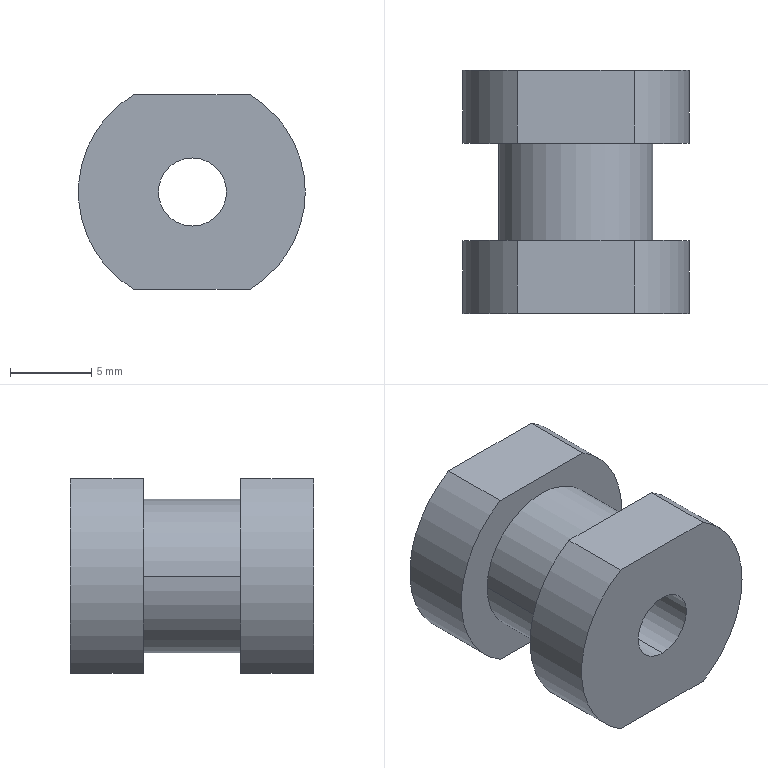Part | STEP file | BU-B05c | 1 solid | 18 faces | box 14 x 15 x 12 mm | volume 1515 mm3 | cylinder 10 | plane 8 | commonest cylinder face diameters 14 x6 4.2 x2 9.5 x2
STEP:
#1=CARTESIAN_POINT('',(0.,0.,0.));
#2=DIRECTION('',(0.,0.,1.));
#3=DIRECTION('',(1.,0.,0.));
#4=AXIS2_PLACEMENT_3D('',#1,#2,#3);
#5=CARTESIAN_POINT('',(0.03736,0.,2.1));
#6=VERTEX_POINT('',#5);
#7=CARTESIAN_POINT('',(0.03736,15.,2.1));
#8=VERTEX_POINT('',#7);
#9=CARTESIAN_POINT('',(0.03736,15.,2.1));
#10=DIRECTION('',(0.,1.,0.));
#11=VECTOR('',#10,1.);
#12=LINE('',#9,#11);
#13=CARTESIAN_POINT('',(0.03736,15.,0.));
#14=DIRECTION('',(0.,1.,0.));
#15=DIRECTION('',(0.,0.,1.));
#16=AXIS2_PLACEMENT_3D('',#13,#14,#15);
#17=CYLINDRICAL_SURFACE('',#16,2.1);
#18=CARTESIAN_POINT('',(6.283,0.));
#19=DIRECTION('',(0.,1.));
#20=VECTOR('',#19,1.);
#21=LINE('',#18,#20);
#22=(GEOMETRIC_REPRESENTATION_CONTEXT(2)PARAMETRIC_REPRESENTATION_CONTEXT()REPRESENTATION_CONTEXT('',''));
#23=DEFINITIONAL_REPRESENTATION('',(#21),#22);
#24=PCURVE('',#17,#23);
#25=CARTESIAN_POINT('',(0.03736,15.,0.));
#26=DIRECTION('',(0.,1.,0.));
#27=DIRECTION('',(0.,0.,1.));
#28=AXIS2_PLACEMENT_3D('',#25,#26,#27);
#29=CYLINDRICAL_SURFACE('',#28,2.1);
#30=CARTESIAN_POINT('',(0.,0.));
#31=DIRECTION('',(0.,1.));
#32=VECTOR('',#31,1.);
#33=LINE('',#30,#32);
#34=(GEOMETRIC_REPRESENTATION_CONTEXT(2)PARAMETRIC_REPRESENTATION_CONTEXT()REPRESENTATION_CONTEXT('',''));
#35=DEFINITIONAL_REPRESENTATION('',(#33),#34);
#36=PCURVE('',#29,#35);
#37=SURFACE_CURVE('',#12,(#24,#36),.PCURVE_S1.);
#38=EDGE_CURVE('',#6,#8,#37,.T.);
#39=ORIENTED_EDGE('',*,*,#38,.T.);
#40=CARTESIAN_POINT('',(0.03736,15.,-2.1));
#41=VERTEX_POINT('',#40);
#42=CARTESIAN_POINT('',(0.03736,15.,0.));
#43=DIRECTION('',(0.,1.,0.));
#44=DIRECTION('',(0.,0.,1.));
#45=AXIS2_PLACEMENT_3D('',#42,#43,#44);
#46=CIRCLE('',#45,2.1);
#47=CARTESIAN_POINT('',(0.,0.));
#48=DIRECTION('',(1.,0.));
#49=VECTOR('',#48,1.);
#50=LINE('',#47,#49);
#51=(GEOMETRIC_REPRESENTATION_CONTEXT(2)PARAMETRIC_REPRESENTATION_CONTEXT()REPRESENTATION_CONTEXT('',''));
#52=DEFINITIONAL_REPRESENTATION('',(#50),#51);
#53=PCURVE('',#17,#52);
#54=CARTESIAN_POINT('',(7.,15.,0.));
#55=DIRECTION('',(0.,1.,0.));
#56=DIRECTION('',(-1.,0.,0.));
#57=AXIS2_PLACEMENT_3D('',#54,#55,#56);
#58=PLANE('',#57);
#59=CARTESIAN_POINT('',(6.963,0.));
#60=DIRECTION('',(0.,1.));
#61=AXIS2_PLACEMENT_2D('',#59,#60);
#62=CIRCLE('',#61,2.1);
#63=(GEOMETRIC_REPRESENTATION_CONTEXT(2)PARAMETRIC_REPRESENTATION_CONTEXT()REPRESENTATION_CONTEXT('',''));
#64=DEFINITIONAL_REPRESENTATION('',(#62),#63);
#65=PCURVE('',#58,#64);
#66=SURFACE_CURVE('',#46,(#53,#65),.PCURVE_S1.);
#67=EDGE_CURVE('',#41,#8,#66,.T.);
#68=ORIENTED_EDGE('',*,*,#67,.F.);
#69=CARTESIAN_POINT('',(0.03736,0.,-2.1));
#70=VERTEX_POINT('',#69);
#71=CARTESIAN_POINT('',(0.03736,15.,-2.1));
#72=DIRECTION('',(0.,1.,0.));
#73=VECTOR('',#72,1.);
#74=LINE('',#71,#73);
#75=CARTESIAN_POINT('',(3.142,0.));
#76=DIRECTION('',(0.,1.));
#77=VECTOR('',#76,1.);
#78=LINE('',#75,#77);
#79=(GEOMETRIC_REPRESENTATION_CONTEXT(2)PARAMETRIC_REPRESENTATION_CONTEXT()REPRESENTATION_CONTEXT('',''));
#80=DEFINITIONAL_REPRESENTATION('',(#78),#79);
#81=PCURVE('',#17,#80);
#82=CARTESIAN_POINT('',(3.142,0.));
#83=DIRECTION('',(0.,1.));
#84=VECTOR('',#83,1.);
#85=LINE('',#82,#84);
#86=(GEOMETRIC_REPRESENTATION_CONTEXT(2)PARAMETRIC_REPRESENTATION_CONTEXT()REPRESENTATION_CONTEXT('',''));
#87=DEFINITIONAL_REPRESENTATION('',(#85),#86);
#88=PCURVE('',#29,#87);
#89=SURFACE_CURVE('',#74,(#81,#88),.PCURVE_S1.);
#90=EDGE_CURVE('',#70,#41,#89,.T.);
#91=ORIENTED_EDGE('',*,*,#90,.F.);
#92=CARTESIAN_POINT('',(0.03736,0.,0.));
#93=DIRECTION('',(0.,1.,0.));
#94=DIRECTION('',(0.,0.,1.));
#95=AXIS2_PLACEMENT_3D('',#92,#93,#94);
#96=CIRCLE('',#95,2.1);
#97=CARTESIAN_POINT('',(0.,-15.));
#98=DIRECTION('',(1.,0.));
#99=VECTOR('',#98,1.);
#100=LINE('',#97,#99);
#101=(GEOMETRIC_REPRESENTATION_CONTEXT(2)PARAMETRIC_REPRESENTATION_CONTEXT()REPRESENTATION_CONTEXT('',''));
#102=DEFINITIONAL_REPRESENTATION('',(#100),#101);
#103=PCURVE('',#17,#102);
#104=CARTESIAN_POINT('',(0.,0.,0.));
#105=DIRECTION('',(0.,-1.,0.));
#106=DIRECTION('',(1.,0.,0.));
#107=AXIS2_PLACEMENT_3D('',#104,#105,#106);
#108=PLANE('',#107);
#109=CARTESIAN_POINT('',(0.03736,2.1));
#110=CARTESIAN_POINT('',(3.675,2.1));
#111=CARTESIAN_POINT('',(1.856,-1.05));
#112=CARTESIAN_POINT('',(0.03736,-4.2));
#113=CARTESIAN_POINT('',(-1.781,-1.05));
#114=CARTESIAN_POINT('',(-3.6,2.1));
#115=CARTESIAN_POINT('',(0.03736,2.1));
#116=(BOUNDED_CURVE()B_SPLINE_CURVE(2,(#109,#110,#111,#112,#113,#114,#115),.UNSPECIFIED.,.T.,.F.)B_SPLINE_CURVE_WITH_KNOTS((1,2,2,2,2,1),(-2.094,0.,2.094,4.189,6.283,8.378),.UNSPECIFIED.)CURVE()GEOMETRIC_REPRESENTATION_ITEM()RATIONAL_B_SPLINE_CURVE((1.,0.5,1.,0.5,1.,0.5,1.))REPRESENTATION_ITEM(''));
#117=(GEOMETRIC_REPRESENTATION_CONTEXT(2)PARAMETRIC_REPRESENTATION_CONTEXT()REPRESENTATION_CONTEXT('',''));
#118=DEFINITIONAL_REPRESENTATION('',(#116),#117);
#119=PCURVE('',#108,#118);
#120=SURFACE_CURVE('',#96,(#103,#119),.PCURVE_S1.);
#121=EDGE_CURVE('',#70,#6,#120,.T.);
#122=ORIENTED_EDGE('',*,*,#121,.T.);
#123=EDGE_LOOP('',(#39,#68,#91,#122));
#124=FACE_BOUND('',#123,.F.);
#125=ADVANCED_FACE('',(#124),#17,.F.);
#126=CARTESIAN_POINT('',(4.75,10.5,0.));
#127=VERTEX_POINT('',#126);
#128=CARTESIAN_POINT('',(-4.75,10.5,0.));
#129=VERTEX_POINT('',#128);
#130=CARTESIAN_POINT('',(0.,10.5,0.));
#131=DIRECTION('',(0.,-1.,0.));
#132=DIRECTION('',(1.,0.,0.));
#133=AXIS2_PLACEMENT_3D('',#130,#131,#132);
#134=CIRCLE('',#133,4.75);
#135=CARTESIAN_POINT('',(0.,-1000.,0.));
#136=DIRECTION('',(0.,-1.,0.));
#137=DIRECTION('',(1.,0.,0.));
#138=AXIS2_PLACEMENT_3D('',#135,#136,#137);
#139=CYLINDRICAL_SURFACE('',#138,4.75);
#140=CARTESIAN_POINT('',(0.,-1010.5));
#141=DIRECTION('',(1.,0.));
#142=VECTOR('',#141,1.);
#143=LINE('',#140,#142);
#144=(GEOMETRIC_REPRESENTATION_CONTEXT(2)PARAMETRIC_REPRESENTATION_CONTEXT()REPRESENTATION_CONTEXT('',''));
#145=DEFINITIONAL_REPRESENTATION('',(#143),#144);
#146=PCURVE('',#139,#145);
#147=CARTESIAN_POINT('',(4.75,10.5,0.));
#148=DIRECTION('',(0.,-1.,0.));
#149=DIRECTION('',(1.,0.,0.));
#150=AXIS2_PLACEMENT_3D('',#147,#148,#149);
#151=PLANE('',#150);
#152=CARTESIAN_POINT('',(-4.75,0.));
#153=DIRECTION('',(1.,0.));
#154=AXIS2_PLACEMENT_2D('',#152,#153);
#155=CIRCLE('',#154,4.75);
#156=(GEOMETRIC_REPRESENTATION_CONTEXT(2)PARAMETRIC_REPRESENTATION_CONTEXT()REPRESENTATION_CONTEXT('',''));
#157=DEFINITIONAL_REPRESENTATION('',(#155),#156);
#158=PCURVE('',#151,#157);
#159=SURFACE_CURVE('',#134,(#146,#158),.PCURVE_S1.);
#160=EDGE_CURVE('',#127,#129,#159,.T.);
#161=ORIENTED_EDGE('',*,*,#160,.T.);
#162=CARTESIAN_POINT('',(-4.75,4.5,0.));
#163=VERTEX_POINT('',#162);
#164=CARTESIAN_POINT('',(-4.75,-1000.,0.));
#165=DIRECTION('',(0.,-1.,0.));
#166=VECTOR('',#165,1.);
#167=LINE('',#164,#166);
#168=CARTESIAN_POINT('',(3.142,0.));
#169=DIRECTION('',(0.,1.));
#170=VECTOR('',#169,1.);
#171=LINE('',#168,#170);
#172=(GEOMETRIC_REPRESENTATION_CONTEXT(2)PARAMETRIC_REPRESENTATION_CONTEXT()REPRESENTATION_CONTEXT('',''));
#173=DEFINITIONAL_REPRESENTATION('',(#171),#172);
#174=PCURVE('',#139,#173);
#175=CARTESIAN_POINT('',(0.,-1000.,0.));
#176=DIRECTION('',(0.,-1.,0.));
#177=DIRECTION('',(1.,0.,0.));
#178=AXIS2_PLACEMENT_3D('',#175,#176,#177);
#179=CYLINDRICAL_SURFACE('',#178,4.75);
#180=CARTESIAN_POINT('',(3.142,0.));
#181=DIRECTION('',(0.,1.));
#182=VECTOR('',#181,1.);
#183=LINE('',#180,#182);
#184=(GEOMETRIC_REPRESENTATION_CONTEXT(2)PARAMETRIC_REPRESENTATION_CONTEXT()REPRESENTATION_CONTEXT('',''));
#185=DEFINITIONAL_REPRESENTATION('',(#183),#184);
#186=PCURVE('',#179,#185);
#187=SURFACE_CURVE('',#167,(#174,#186),.PCURVE_S1.);
#188=EDGE_CURVE('',#129,#163,#187,.T.);
#189=ORIENTED_EDGE('',*,*,#188,.T.);
#190=CARTESIAN_POINT('',(4.75,4.5,0.));
#191=VERTEX_POINT('',#190);
#192=CARTESIAN_POINT('',(0.,4.5,0.));
#193=DIRECTION('',(0.,-1.,0.));
#194=DIRECTION('',(1.,0.,0.));
#195=AXIS2_PLACEMENT_3D('',#192,#193,#194);
#196=CIRCLE('',#195,4.75);
#197=CARTESIAN_POINT('',(0.,-1004.5));
#198=DIRECTION('',(1.,0.));
#199=VECTOR('',#198,1.);
#200=LINE('',#197,#199);
#201=(GEOMETRIC_REPRESENTATION_CONTEXT(2)PARAMETRIC_REPRESENTATION_CONTEXT()REPRESENTATION_CONTEXT('',''));
#202=DEFINITIONAL_REPRESENTATION('',(#200),#201);
#203=PCURVE('',#139,#202);
#204=CARTESIAN_POINT('',(7.,4.5,0.));
#205=DIRECTION('',(0.,1.,0.));
#206=DIRECTION('',(-1.,0.,0.));
#207=AXIS2_PLACEMENT_3D('',#204,#205,#206);
#208=PLANE('',#207);
#209=CARTESIAN_POINT('',(2.25,0.));
#210=CARTESIAN_POINT('',(2.25,8.227));
#211=CARTESIAN_POINT('',(9.375,4.114));
#212=CARTESIAN_POINT('',(16.5,0.));
#213=CARTESIAN_POINT('',(9.375,-4.114));
#214=CARTESIAN_POINT('',(2.25,-8.227));
#215=CARTESIAN_POINT('',(2.25,0.));
#216=(BOUNDED_CURVE()B_SPLINE_CURVE(2,(#209,#210,#211,#212,#213,#214,#215),.UNSPECIFIED.,.T.,.F.)B_SPLINE_CURVE_WITH_KNOTS((1,2,2,2,2,1),(-2.094,0.,2.094,4.189,6.283,8.378),.UNSPECIFIED.)CURVE()GEOMETRIC_REPRESENTATION_ITEM()RATIONAL_B_SPLINE_CURVE((1.,0.5,1.,0.5,1.,0.5,1.))REPRESENTATION_ITEM(''));
#217=(GEOMETRIC_REPRESENTATION_CONTEXT(2)PARAMETRIC_REPRESENTATION_CONTEXT()REPRESENTATION_CONTEXT('',''));
#218=DEFINITIONAL_REPRESENTATION('',(#216),#217);
#219=PCURVE('',#208,#218);
#220=SURFACE_CURVE('',#196,(#203,#219),.PCURVE_S1.);
#221=EDGE_CURVE('',#191,#163,#220,.T.);
#222=ORIENTED_EDGE('',*,*,#221,.F.);
#223=CARTESIAN_POINT('',(4.75,-1000.,0.));
#224=DIRECTION('',(0.,-1.,0.));
#225=VECTOR('',#224,1.);
#226=LINE('',#223,#225);
#227=CARTESIAN_POINT('',(0.,0.));
#228=DIRECTION('',(0.,1.));
#229=VECTOR('',#228,1.);
#230=LINE('',#227,#229);
#231=(GEOMETRIC_REPRESENTATION_CONTEXT(2)PARAMETRIC_REPRESENTATION_CONTEXT()REPRESENTATION_CONTEXT('',''));
#232=DEFINITIONAL_REPRESENTATION('',(#230),#231);
#233=PCURVE('',#139,#232);
#234=CARTESIAN_POINT('',(6.283,0.));
#235=DIRECTION('',(0.,1.));
#236=VECTOR('',#235,1.);
#237=LINE('',#234,#236);
#238=(GEOMETRIC_REPRESENTATION_CONTEXT(2)PARAMETRIC_REPRESENTATION_CONTEXT()REPRESENTATION_CONTEXT('',''));
#239=DEFINITIONAL_REPRESENTATION('',(#237),#238);
#240=PCURVE('',#179,#239);
#241=SURFACE_CURVE('',#226,(#233,#240),.PCURVE_S1.);
#242=EDGE_CURVE('',#127,#191,#241,.T.);
#243=ORIENTED_EDGE('',*,*,#242,.F.);
#244=EDGE_LOOP('',(#161,#189,#222,#243));
#245=FACE_BOUND('',#244,.T.);
#246=ADVANCED_FACE('',(#245),#139,.T.);
#247=CARTESIAN_POINT('',(3.606,15.,-6.));
#248=VERTEX_POINT('',#247);
#249=CARTESIAN_POINT('',(7.,15.,0.));
#250=VERTEX_POINT('',#249);
#251=CARTESIAN_POINT('',(0.,15.,0.));
#252=DIRECTION('',(0.,-1.,0.));
#253=DIRECTION('',(1.,0.,0.));
#254=AXIS2_PLACEMENT_3D('',#251,#252,#253);
#255=CIRCLE('',#254,7.);
#256=CARTESIAN_POINT('',(0.,-1000.,0.));
#257=DIRECTION('',(0.,-1.,0.));
#258=DIRECTION('',(1.,0.,0.));
#259=AXIS2_PLACEMENT_3D('',#256,#257,#258);
#260=CYLINDRICAL_SURFACE('',#259,7.);
#261=CARTESIAN_POINT('',(0.,-1015.));
#262=DIRECTION('',(1.,0.));
#263=VECTOR('',#262,1.);
#264=LINE('',#261,#263);
#265=(GEOMETRIC_REPRESENTATION_CONTEXT(2)PARAMETRIC_REPRESENTATION_CONTEXT()REPRESENTATION_CONTEXT('',''));
#266=DEFINITIONAL_REPRESENTATION('',(#264),#265);
#267=PCURVE('',#260,#266);
#268=CARTESIAN_POINT('',(0.,0.));
#269=CARTESIAN_POINT('',(0.,12.124));
#270=CARTESIAN_POINT('',(10.5,6.062));
#271=CARTESIAN_POINT('',(21.,0.));
#272=CARTESIAN_POINT('',(10.5,-6.062));
#273=CARTESIAN_POINT('',(0.,-12.124));
#274=CARTESIAN_POINT('',(0.,0.));
#275=(BOUNDED_CURVE()B_SPLINE_CURVE(2,(#268,#269,#270,#271,#272,#273,#274),.UNSPECIFIED.,.T.,.F.)B_SPLINE_CURVE_WITH_KNOTS((1,2,2,2,2,1),(-2.094,0.,2.094,4.189,6.283,8.378),.UNSPECIFIED.)CURVE()GEOMETRIC_REPRESENTATION_ITEM()RATIONAL_B_SPLINE_CURVE((1.,0.5,1.,0.5,1.,0.5,1.))REPRESENTATION_ITEM(''));
#276=(GEOMETRIC_REPRESENTATION_CONTEXT(2)PARAMETRIC_REPRESENTATION_CONTEXT()REPRESENTATION_CONTEXT('',''));
#277=DEFINITIONAL_REPRESENTATION('',(#275),#276);
#278=PCURVE('',#58,#277);
#279=SURFACE_CURVE('',#255,(#267,#278),.PCURVE_S1.);
#280=EDGE_CURVE('',#248,#250,#279,.T.);
#281=ORIENTED_EDGE('',*,*,#280,.T.);
#282=CARTESIAN_POINT('',(7.,10.5,0.));
#283=VERTEX_POINT('',#282);
#284=CARTESIAN_POINT('',(7.,-1000.,0.));
#285=DIRECTION('',(0.,-1.,0.));
#286=VECTOR('',#285,1.);
#287=LINE('',#284,#286);
#288=CARTESIAN_POINT('',(6.283,0.));
#289=DIRECTION('',(0.,1.));
#290=VECTOR('',#289,1.);
#291=LINE('',#288,#290);
#292=(GEOMETRIC_REPRESENTATION_CONTEXT(2)PARAMETRIC_REPRESENTATION_CONTEXT()REPRESENTATION_CONTEXT('',''));
#293=DEFINITIONAL_REPRESENTATION('',(#291),#292);
#294=PCURVE('',#260,#293);
#295=CARTESIAN_POINT('',(0.,-1000.,0.));
#296=DIRECTION('',(0.,-1.,0.));
#297=DIRECTION('',(1.,0.,0.));
#298=AXIS2_PLACEMENT_3D('',#295,#296,#297);
#299=CYLINDRICAL_SURFACE('',#298,7.);
#300=CARTESIAN_POINT('',(0.,0.));
#301=DIRECTION('',(0.,1.));
#302=VECTOR('',#301,1.);
#303=LINE('',#300,#302);
#304=(GEOMETRIC_REPRESENTATION_CONTEXT(2)PARAMETRIC_REPRESENTATION_CONTEXT()REPRESENTATION_CONTEXT('',''));
#305=DEFINITIONAL_REPRESENTATION('',(#303),#304);
#306=PCURVE('',#299,#305);
#307=SURFACE_CURVE('',#287,(#294,#306),.PCURVE_S1.);
#308=EDGE_CURVE('',#250,#283,#307,.T.);
#309=ORIENTED_EDGE('',*,*,#308,.T.);
#310=CARTESIAN_POINT('',(3.606,10.5,-6.));
#311=VERTEX_POINT('',#310);
#312=CARTESIAN_POINT('',(0.,10.5,0.));
#313=DIRECTION('',(0.,-1.,0.));
#314=DIRECTION('',(1.,0.,0.));
#315=AXIS2_PLACEMENT_3D('',#312,#313,#314);
#316=CIRCLE('',#315,7.);
#317=CARTESIAN_POINT('',(0.,-1010.5));
#318=DIRECTION('',(1.,0.));
#319=VECTOR('',#318,1.);
#320=LINE('',#317,#319);
#321=(GEOMETRIC_REPRESENTATION_CONTEXT(2)PARAMETRIC_REPRESENTATION_CONTEXT()REPRESENTATION_CONTEXT('',''));
#322=DEFINITIONAL_REPRESENTATION('',(#320),#321);
#323=PCURVE('',#260,#322);
#324=CARTESIAN_POINT('',(-4.75,0.));
#325=DIRECTION('',(1.,0.));
#326=AXIS2_PLACEMENT_2D('',#324,#325);
#327=CIRCLE('',#326,7.);
#328=(GEOMETRIC_REPRESENTATION_CONTEXT(2)PARAMETRIC_REPRESENTATION_CONTEXT()REPRESENTATION_CONTEXT('',''));
#329=DEFINITIONAL_REPRESENTATION('',(#327),#328);
#330=PCURVE('',#151,#329);
#331=SURFACE_CURVE('',#316,(#323,#330),.PCURVE_S1.);
#332=EDGE_CURVE('',#311,#283,#331,.T.);
#333=ORIENTED_EDGE('',*,*,#332,.F.);
#334=CARTESIAN_POINT('',(3.606,0.,-6.));
#335=DIRECTION('',(0.,1.,0.));
#336=VECTOR('',#335,1.);
#337=LINE('',#334,#336);
#338=CARTESIAN_POINT('',(5.253,-1000.));
#339=DIRECTION('',(0.,-1.));
#340=VECTOR('',#339,1.);
#341=LINE('',#338,#340);
#342=(GEOMETRIC_REPRESENTATION_CONTEXT(2)PARAMETRIC_REPRESENTATION_CONTEXT()REPRESENTATION_CONTEXT('',''));
#343=DEFINITIONAL_REPRESENTATION('',(#341),#342);
#344=PCURVE('',#260,#343);
#345=CARTESIAN_POINT('',(-3.606,0.,-6.));
#346=DIRECTION('',(0.,0.,1.));
#347=DIRECTION('',(1.,0.,0.));
#348=AXIS2_PLACEMENT_3D('',#345,#346,#347);
#349=PLANE('',#348);
#350=CARTESIAN_POINT('',(7.211,0.));
#351=DIRECTION('',(0.,1.));
#352=VECTOR('',#351,1.);
#353=LINE('',#350,#352);
#354=(GEOMETRIC_REPRESENTATION_CONTEXT(2)PARAMETRIC_REPRESENTATION_CONTEXT()REPRESENTATION_CONTEXT('',''));
#355=DEFINITIONAL_REPRESENTATION('',(#353),#354);
#356=PCURVE('',#349,#355);
#357=SURFACE_CURVE('',#337,(#344,#356),.PCURVE_S1.);
#358=EDGE_CURVE('',#311,#248,#357,.T.);
#359=ORIENTED_EDGE('',*,*,#358,.T.);
#360=EDGE_LOOP('',(#281,#309,#333,#359));
#361=FACE_BOUND('',#360,.T.);
#362=ADVANCED_FACE('',(#361),#260,.T.);
#363=CARTESIAN_POINT('',(3.606,4.5,-6.));
#364=VERTEX_POINT('',#363);
#365=CARTESIAN_POINT('',(7.,4.5,0.));
#366=VERTEX_POINT('',#365);
#367=CARTESIAN_POINT('',(0.,4.5,0.));
#368=DIRECTION('',(0.,-1.,0.));
#369=DIRECTION('',(1.,0.,0.));
#370=AXIS2_PLACEMENT_3D('',#367,#368,#369);
#371=CIRCLE('',#370,7.);
#372=CARTESIAN_POINT('',(0.,-1000.,0.));
#373=DIRECTION('',(0.,-1.,0.));
#374=DIRECTION('',(1.,0.,0.));
#375=AXIS2_PLACEMENT_3D('',#372,#373,#374);
#376=CYLINDRICAL_SURFACE('',#375,7.);
#377=CARTESIAN_POINT('',(0.,-1004.5));
#378=DIRECTION('',(1.,0.));
#379=VECTOR('',#378,1.);
#380=LINE('',#377,#379);
#381=(GEOMETRIC_REPRESENTATION_CONTEXT(2)PARAMETRIC_REPRESENTATION_CONTEXT()REPRESENTATION_CONTEXT('',''));
#382=DEFINITIONAL_REPRESENTATION('',(#380),#381);
#383=PCURVE('',#376,#382);
#384=CARTESIAN_POINT('',(0.,0.));
#385=CARTESIAN_POINT('',(0.,12.124));
#386=CARTESIAN_POINT('',(10.5,6.062));
#387=CARTESIAN_POINT('',(21.,0.));
#388=CARTESIAN_POINT('',(10.5,-6.062));
#389=CARTESIAN_POINT('',(0.,-12.124));
#390=CARTESIAN_POINT('',(0.,0.));
#391=(BOUNDED_CURVE()B_SPLINE_CURVE(2,(#384,#385,#386,#387,#388,#389,#390),.UNSPECIFIED.,.T.,.F.)B_SPLINE_CURVE_WITH_KNOTS((1,2,2,2,2,1),(-2.094,0.,2.094,4.189,6.283,8.378),.UNSPECIFIED.)CURVE()GEOMETRIC_REPRESENTATION_ITEM()RATIONAL_B_SPLINE_CURVE((1.,0.5,1.,0.5,1.,0.5,1.))REPRESENTATION_ITEM(''));
#392=(GEOMETRIC_REPRESENTATION_CONTEXT(2)PARAMETRIC_REPRESENTATION_CONTEXT()REPRESENTATION_CONTEXT('',''));
#393=DEFINITIONAL_REPRESENTATION('',(#391),#392);
#394=PCURVE('',#208,#393);
#395=SURFACE_CURVE('',#371,(#383,#394),.PCURVE_S1.);
#396=EDGE_CURVE('',#364,#366,#395,.T.);
#397=ORIENTED_EDGE('',*,*,#396,.T.);
#398=CARTESIAN_POINT('',(7.,0.,0.));
#399=VERTEX_POINT('',#398);
#400=CARTESIAN_POINT('',(7.,-1000.,0.));
#401=DIRECTION('',(0.,-1.,0.));
#402=VECTOR('',#401,1.);
#403=LINE('',#400,#402);
#404=CARTESIAN_POINT('',(6.283,0.));
#405=DIRECTION('',(0.,1.));
#406=VECTOR('',#405,1.);
#407=LINE('',#404,#406);
#408=(GEOMETRIC_REPRESENTATION_CONTEXT(2)PARAMETRIC_REPRESENTATION_CONTEXT()REPRESENTATION_CONTEXT('',''));
#409=DEFINITIONAL_REPRESENTATION('',(#407),#408);
#410=PCURVE('',#376,#409);
#411=CARTESIAN_POINT('',(0.,-1000.,0.));
#412=DIRECTION('',(0.,-1.,0.));
#413=DIRECTION('',(1.,0.,0.));
#414=AXIS2_PLACEMENT_3D('',#411,#412,#413);
#415=CYLINDRICAL_SURFACE('',#414,7.);
#416=CARTESIAN_POINT('',(0.,0.));
#417=DIRECTION('',(0.,1.));
#418=VECTOR('',#417,1.);
#419=LINE('',#416,#418);
#420=(GEOMETRIC_REPRESENTATION_CONTEXT(2)PARAMETRIC_REPRESENTATION_CONTEXT()REPRESENTATION_CONTEXT('',''));
#421=DEFINITIONAL_REPRESENTATION('',(#419),#420);
#422=PCURVE('',#415,#421);
#423=SURFACE_CURVE('',#403,(#410,#422),.PCURVE_S1.);
#424=EDGE_CURVE('',#366,#399,#423,.T.);
#425=ORIENTED_EDGE('',*,*,#424,.T.);
#426=CARTESIAN_POINT('',(3.606,0.,-6.));
#427=VERTEX_POINT('',#426);
#428=CARTESIAN_POINT('',(0.,0.,0.));
#429=DIRECTION('',(0.,-1.,0.));
#430=DIRECTION('',(1.,0.,0.));
#431=AXIS2_PLACEMENT_3D('',#428,#429,#430);
#432=CIRCLE('',#431,7.);
#433=CARTESIAN_POINT('',(0.,-1000.));
#434=DIRECTION('',(1.,0.));
#435=VECTOR('',#434,1.);
#436=LINE('',#433,#435);
#437=(GEOMETRIC_REPRESENTATION_CONTEXT(2)PARAMETRIC_REPRESENTATION_CONTEXT()REPRESENTATION_CONTEXT('',''));
#438=DEFINITIONAL_REPRESENTATION('',(#436),#437);
#439=PCURVE('',#376,#438);
#440=CARTESIAN_POINT('',(0.,0.));
#441=DIRECTION('',(1.,0.));
#442=AXIS2_PLACEMENT_2D('',#440,#441);
#443=CIRCLE('',#442,7.);
#444=(GEOMETRIC_REPRESENTATION_CONTEXT(2)PARAMETRIC_REPRESENTATION_CONTEXT()REPRESENTATION_CONTEXT('',''));
#445=DEFINITIONAL_REPRESENTATION('',(#443),#444);
#446=PCURVE('',#108,#445);
#447=SURFACE_CURVE('',#432,(#439,#446),.PCURVE_S1.);
#448=EDGE_CURVE('',#427,#399,#447,.T.);
#449=ORIENTED_EDGE('',*,*,#448,.F.);
#450=CARTESIAN_POINT('',(3.606,0.,-6.));
#451=DIRECTION('',(0.,1.,0.));
#452=VECTOR('',#451,1.);
#453=LINE('',#450,#452);
#454=CARTESIAN_POINT('',(5.253,-1000.));
#455=DIRECTION('',(0.,-1.));
#456=VECTOR('',#455,1.);
#457=LINE('',#454,#456);
#458=(GEOMETRIC_REPRESENTATION_CONTEXT(2)PARAMETRIC_REPRESENTATION_CONTEXT()REPRESENTATION_CONTEXT('',''));
#459=DEFINITIONAL_REPRESENTATION('',(#457),#458);
#460=PCURVE('',#376,#459);
#461=CARTESIAN_POINT('',(-3.606,0.,-6.));
#462=DIRECTION('',(0.,0.,1.));
#463=DIRECTION('',(1.,0.,0.));
#464=AXIS2_PLACEMENT_3D('',#461,#462,#463);
#465=PLANE('',#464);
#466=CARTESIAN_POINT('',(7.211,0.));
#467=DIRECTION('',(0.,1.));
#468=VECTOR('',#467,1.);
#469=LINE('',#466,#468);
#470=(GEOMETRIC_REPRESENTATION_CONTEXT(2)PARAMETRIC_REPRESENTATION_CONTEXT()REPRESENTATION_CONTEXT('',''));
#471=DEFINITIONAL_REPRESENTATION('',(#469),#470);
#472=PCURVE('',#465,#471);
#473=SURFACE_CURVE('',#453,(#460,#472),.PCURVE_S1.);
#474=EDGE_CURVE('',#427,#364,#473,.T.);
#475=ORIENTED_EDGE('',*,*,#474,.T.);
#476=EDGE_LOOP('',(#397,#425,#449,#475));
#477=FACE_BOUND('',#476,.T.);
#478=ADVANCED_FACE('',(#477),#376,.T.);
#479=ORIENTED_EDGE('',*,*,#424,.F.);
#480=CARTESIAN_POINT('',(3.606,4.5,6.));
#481=VERTEX_POINT('',#480);
#482=CARTESIAN_POINT('',(0.,4.5,0.));
#483=DIRECTION('',(0.,-1.,0.));
#484=DIRECTION('',(1.,0.,0.));
#485=AXIS2_PLACEMENT_3D('',#482,#483,#484);
#486=CIRCLE('',#485,7.);
#487=CARTESIAN_POINT('',(0.,-1004.5));
#488=DIRECTION('',(1.,0.));
#489=VECTOR('',#488,1.);
#490=LINE('',#487,#489);
#491=(GEOMETRIC_REPRESENTATION_CONTEXT(2)PARAMETRIC_REPRESENTATION_CONTEXT()REPRESENTATION_CONTEXT('',''));
#492=DEFINITIONAL_REPRESENTATION('',(#490),#491);
#493=PCURVE('',#415,#492);
#494=CARTESIAN_POINT('',(0.,0.));
#495=CARTESIAN_POINT('',(0.,12.124));
#496=CARTESIAN_POINT('',(10.5,6.062));
#497=CARTESIAN_POINT('',(21.,0.));
#498=CARTESIAN_POINT('',(10.5,-6.062));
#499=CARTESIAN_POINT('',(0.,-12.124));
#500=CARTESIAN_POINT('',(0.,0.));
#501=(BOUNDED_CURVE()B_SPLINE_CURVE(2,(#494,#495,#496,#497,#498,#499,#500),.UNSPECIFIED.,.T.,.F.)B_SPLINE_CURVE_WITH_KNOTS((1,2,2,2,2,1),(-2.094,0.,2.094,4.189,6.283,8.378),.UNSPECIFIED.)CURVE()GEOMETRIC_REPRESENTATION_ITEM()RATIONAL_B_SPLINE_CURVE((1.,0.5,1.,0.5,1.,0.5,1.))REPRESENTATION_ITEM(''));
#502=(GEOMETRIC_REPRESENTATION_CONTEXT(2)PARAMETRIC_REPRESENTATION_CONTEXT()REPRESENTATION_CONTEXT('',''));
#503=DEFINITIONAL_REPRESENTATION('',(#501),#502);
#504=PCURVE('',#208,#503);
#505=SURFACE_CURVE('',#486,(#493,#504),.PCURVE_S1.);
#506=EDGE_CURVE('',#366,#481,#505,.T.);
#507=ORIENTED_EDGE('',*,*,#506,.T.);
#508=CARTESIAN_POINT('',(3.606,0.,6.));
#509=VERTEX_POINT('',#508);
#510=CARTESIAN_POINT('',(3.606,0.,6.));
#511=DIRECTION('',(0.,1.,0.));
#512=VECTOR('',#511,1.);
#513=LINE('',#510,#512);
#514=CARTESIAN_POINT('',(1.03,-1000.));
#515=DIRECTION('',(0.,-1.));
#516=VECTOR('',#515,1.);
#517=LINE('',#514,#516);
#518=(GEOMETRIC_REPRESENTATION_CONTEXT(2)PARAMETRIC_REPRESENTATION_CONTEXT()REPRESENTATION_CONTEXT('',''));
#519=DEFINITIONAL_REPRESENTATION('',(#517),#518);
#520=PCURVE('',#415,#519);
#521=CARTESIAN_POINT('',(-3.606,0.,6.));
#522=DIRECTION('',(0.,0.,-1.));
#523=DIRECTION('',(-1.,0.,0.));
#524=AXIS2_PLACEMENT_3D('',#521,#522,#523);
#525=PLANE('',#524);
#526=CARTESIAN_POINT('',(-7.211,0.));
#527=DIRECTION('',(0.,1.));
#528=VECTOR('',#527,1.);
#529=LINE('',#526,#528);
#530=(GEOMETRIC_REPRESENTATION_CONTEXT(2)PARAMETRIC_REPRESENTATION_CONTEXT()REPRESENTATION_CONTEXT('',''));
#531=DEFINITIONAL_REPRESENTATION('',(#529),#530);
#532=PCURVE('',#525,#531);
#533=SURFACE_CURVE('',#513,(#520,#532),.PCURVE_S1.);
#534=EDGE_CURVE('',#509,#481,#533,.T.);
#535=ORIENTED_EDGE('',*,*,#534,.F.);
#536=CARTESIAN_POINT('',(0.,0.,0.));
#537=DIRECTION('',(0.,-1.,0.));
#538=DIRECTION('',(1.,0.,0.));
#539=AXIS2_PLACEMENT_3D('',#536,#537,#538);
#540=CIRCLE('',#539,7.);
#541=CARTESIAN_POINT('',(0.,-1000.));
#542=DIRECTION('',(1.,0.));
#543=VECTOR('',#542,1.);
#544=LINE('',#541,#543);
#545=(GEOMETRIC_REPRESENTATION_CONTEXT(2)PARAMETRIC_REPRESENTATION_CONTEXT()REPRESENTATION_CONTEXT('',''));
#546=DEFINITIONAL_REPRESENTATION('',(#544),#545);
#547=PCURVE('',#415,#546);
#548=CARTESIAN_POINT('',(0.,0.));
#549=DIRECTION('',(1.,0.));
#550=AXIS2_PLACEMENT_2D('',#548,#549);
#551=CIRCLE('',#550,7.);
#552=(GEOMETRIC_REPRESENTATION_CONTEXT(2)PARAMETRIC_REPRESENTATION_CONTEXT()REPRESENTATION_CONTEXT('',''));
#553=DEFINITIONAL_REPRESENTATION('',(#551),#552);
#554=PCURVE('',#108,#553);
#555=SURFACE_CURVE('',#540,(#547,#554),.PCURVE_S1.);
#556=EDGE_CURVE('',#399,#509,#555,.T.);
#557=ORIENTED_EDGE('',*,*,#556,.F.);
#558=EDGE_LOOP('',(#479,#507,#535,#557));
#559=FACE_BOUND('',#558,.T.);
#560=ADVANCED_FACE('',(#559),#415,.T.);
#561=ORIENTED_EDGE('',*,*,#308,.F.);
#562=CARTESIAN_POINT('',(3.606,15.,6.));
#563=VERTEX_POINT('',#562);
#564=CARTESIAN_POINT('',(0.,15.,0.));
#565=DIRECTION('',(0.,-1.,0.));
#566=DIRECTION('',(1.,0.,0.));
#567=AXIS2_PLACEMENT_3D('',#564,#565,#566);
#568=CIRCLE('',#567,7.);
#569=CARTESIAN_POINT('',(0.,-1015.));
#570=DIRECTION('',(1.,0.));
#571=VECTOR('',#570,1.);
#572=LINE('',#569,#571);
#573=(GEOMETRIC_REPRESENTATION_CONTEXT(2)PARAMETRIC_REPRESENTATION_CONTEXT()REPRESENTATION_CONTEXT('',''));
#574=DEFINITIONAL_REPRESENTATION('',(#572),#573);
#575=PCURVE('',#299,#574);
#576=CARTESIAN_POINT('',(0.,0.));
#577=CARTESIAN_POINT('',(0.,12.124));
#578=CARTESIAN_POINT('',(10.5,6.062));
#579=CARTESIAN_POINT('',(21.,0.));
#580=CARTESIAN_POINT('',(10.5,-6.062));
#581=CARTESIAN_POINT('',(0.,-12.124));
#582=CARTESIAN_POINT('',(0.,0.));
#583=(BOUNDED_CURVE()B_SPLINE_CURVE(2,(#576,#577,#578,#579,#580,#581,#582),.UNSPECIFIED.,.T.,.F.)B_SPLINE_CURVE_WITH_KNOTS((1,2,2,2,2,1),(-2.094,0.,2.094,4.189,6.283,8.378),.UNSPECIFIED.)CURVE()GEOMETRIC_REPRESENTATION_ITEM()RATIONAL_B_SPLINE_CURVE((1.,0.5,1.,0.5,1.,0.5,1.))REPRESENTATION_ITEM(''));
#584=(GEOMETRIC_REPRESENTATION_CONTEXT(2)PARAMETRIC_REPRESENTATION_CONTEXT()REPRESENTATION_CONTEXT('',''));
#585=DEFINITIONAL_REPRESENTATION('',(#583),#584);
#586=PCURVE('',#58,#585);
#587=SURFACE_CURVE('',#568,(#575,#586),.PCURVE_S1.);
#588=EDGE_CURVE('',#250,#563,#587,.T.);
#589=ORIENTED_EDGE('',*,*,#588,.T.);
#590=CARTESIAN_POINT('',(3.606,10.5,6.));
#591=VERTEX_POINT('',#590);
#592=CARTESIAN_POINT('',(3.606,0.,6.));
#593=DIRECTION('',(0.,1.,0.));
#594=VECTOR('',#593,1.);
#595=LINE('',#592,#594);
#596=CARTESIAN_POINT('',(1.03,-1000.));
#597=DIRECTION('',(0.,-1.));
#598=VECTOR('',#597,1.);
#599=LINE('',#596,#598);
#600=(GEOMETRIC_REPRESENTATION_CONTEXT(2)PARAMETRIC_REPRESENTATION_CONTEXT()REPRESENTATION_CONTEXT('',''));
#601=DEFINITIONAL_REPRESENTATION('',(#599),#600);
#602=PCURVE('',#299,#601);
#603=CARTESIAN_POINT('',(-3.606,0.,6.));
#604=DIRECTION('',(0.,0.,-1.));
#605=DIRECTION('',(-1.,0.,0.));
#606=AXIS2_PLACEMENT_3D('',#603,#604,#605);
#607=PLANE('',#606);
#608=CARTESIAN_POINT('',(-7.211,0.));
#609=DIRECTION('',(0.,1.));
#610=VECTOR('',#609,1.);
#611=LINE('',#608,#610);
#612=(GEOMETRIC_REPRESENTATION_CONTEXT(2)PARAMETRIC_REPRESENTATION_CONTEXT()REPRESENTATION_CONTEXT('',''));
#613=DEFINITIONAL_REPRESENTATION('',(#611),#612);
#614=PCURVE('',#607,#613);
#615=SURFACE_CURVE('',#595,(#602,#614),.PCURVE_S1.);
#616=EDGE_CURVE('',#591,#563,#615,.T.);
#617=ORIENTED_EDGE('',*,*,#616,.F.);
#618=CARTESIAN_POINT('',(0.,10.5,0.));
#619=DIRECTION('',(0.,-1.,0.));
#620=DIRECTION('',(1.,0.,0.));
#621=AXIS2_PLACEMENT_3D('',#618,#619,#620);
#622=CIRCLE('',#621,7.);
#623=CARTESIAN_POINT('',(0.,-1010.5));
#624=DIRECTION('',(1.,0.));
#625=VECTOR('',#624,1.);
#626=LINE('',#623,#625);
#627=(GEOMETRIC_REPRESENTATION_CONTEXT(2)PARAMETRIC_REPRESENTATION_CONTEXT()REPRESENTATION_CONTEXT('',''));
#628=DEFINITIONAL_REPRESENTATION('',(#626),#627);
#629=PCURVE('',#299,#628);
#630=CARTESIAN_POINT('',(-4.75,0.));
#631=DIRECTION('',(1.,0.));
#632=AXIS2_PLACEMENT_2D('',#630,#631);
#633=CIRCLE('',#632,7.);
#634=(GEOMETRIC_REPRESENTATION_CONTEXT(2)PARAMETRIC_REPRESENTATION_CONTEXT()REPRESENTATION_CONTEXT('',''));
#635=DEFINITIONAL_REPRESENTATION('',(#633),#634);
#636=PCURVE('',#151,#635);
#637=SURFACE_CURVE('',#622,(#629,#636),.PCURVE_S1.);
#638=EDGE_CURVE('',#283,#591,#637,.T.);
#639=ORIENTED_EDGE('',*,*,#638,.F.);
#640=EDGE_LOOP('',(#561,#589,#617,#639));
#641=FACE_BOUND('',#640,.T.);
#642=ADVANCED_FACE('',(#641),#299,.T.);
#643=CARTESIAN_POINT('',(0.03736,0.,0.));
#644=DIRECTION('',(0.,1.,0.));
#645=DIRECTION('',(0.,0.,1.));
#646=AXIS2_PLACEMENT_3D('',#643,#644,#645);
#647=CIRCLE('',#646,2.1);
#648=CARTESIAN_POINT('',(0.03736,2.1));
#649=CARTESIAN_POINT('',(3.675,2.1));
#650=CARTESIAN_POINT('',(1.856,-1.05));
#651=CARTESIAN_POINT('',(0.03736,-4.2));
#652=CARTESIAN_POINT('',(-1.781,-1.05));
#653=CARTESIAN_POINT('',(-3.6,2.1));
#654=CARTESIAN_POINT('',(0.03736,2.1));
#655=(BOUNDED_CURVE()B_SPLINE_CURVE(2,(#648,#649,#650,#651,#652,#653,#654),.UNSPECIFIED.,.T.,.F.)B_SPLINE_CURVE_WITH_KNOTS((1,2,2,2,2,1),(-2.094,0.,2.094,4.189,6.283,8.378),.UNSPECIFIED.)CURVE()GEOMETRIC_REPRESENTATION_ITEM()RATIONAL_B_SPLINE_CURVE((1.,0.5,1.,0.5,1.,0.5,1.))REPRESENTATION_ITEM(''));
#656=(GEOMETRIC_REPRESENTATION_CONTEXT(2)PARAMETRIC_REPRESENTATION_CONTEXT()REPRESENTATION_CONTEXT('',''));
#657=DEFINITIONAL_REPRESENTATION('',(#655),#656);
#658=PCURVE('',#108,#657);
#659=CARTESIAN_POINT('',(0.,-15.));
#660=DIRECTION('',(1.,0.));
#661=VECTOR('',#660,1.);
#662=LINE('',#659,#661);
#663=(GEOMETRIC_REPRESENTATION_CONTEXT(2)PARAMETRIC_REPRESENTATION_CONTEXT()REPRESENTATION_CONTEXT('',''));
#664=DEFINITIONAL_REPRESENTATION('',(#662),#663);
#665=PCURVE('',#29,#664);
#666=SURFACE_CURVE('',#647,(#658,#665),.PCURVE_S1.);
#667=EDGE_CURVE('',#6,#70,#666,.T.);
#668=ORIENTED_EDGE('',*,*,#667,.T.);
#669=ORIENTED_EDGE('',*,*,#121,.T.);
#670=EDGE_LOOP('',(#668,#669));
#671=FACE_BOUND('',#670,.T.);
#672=CARTESIAN_POINT('',(-3.606,0.,6.));
#673=VERTEX_POINT('',#672);
#674=CARTESIAN_POINT('',(-3.606,0.,6.));
#675=DIRECTION('',(-1.,0.,0.));
#676=VECTOR('',#675,1.);
#677=LINE('',#674,#676);
#678=CARTESIAN_POINT('',(-3.606,6.));
#679=DIRECTION('',(-1.,0.));
#680=VECTOR('',#679,1.);
#681=LINE('',#678,#680);
#682=(GEOMETRIC_REPRESENTATION_CONTEXT(2)PARAMETRIC_REPRESENTATION_CONTEXT()REPRESENTATION_CONTEXT('',''));
#683=DEFINITIONAL_REPRESENTATION('',(#681),#682);
#684=PCURVE('',#108,#683);
#685=CARTESIAN_POINT('',(0.,0.));
#686=DIRECTION('',(1.,0.));
#687=VECTOR('',#686,1.);
#688=LINE('',#685,#687);
#689=(GEOMETRIC_REPRESENTATION_CONTEXT(2)PARAMETRIC_REPRESENTATION_CONTEXT()REPRESENTATION_CONTEXT('',''));
#690=DEFINITIONAL_REPRESENTATION('',(#688),#689);
#691=PCURVE('',#525,#690);
#692=SURFACE_CURVE('',#677,(#684,#691),.PCURVE_S1.);
#693=EDGE_CURVE('',#509,#673,#692,.T.);
#694=ORIENTED_EDGE('',*,*,#693,.T.);
#695=CARTESIAN_POINT('',(-3.606,0.,-6.));
#696=VERTEX_POINT('',#695);
#697=CARTESIAN_POINT('',(0.,0.,0.));
#698=DIRECTION('',(0.,-1.,0.));
#699=DIRECTION('',(1.,0.,0.));
#700=AXIS2_PLACEMENT_3D('',#697,#698,#699);
#701=CIRCLE('',#700,7.);
#702=CARTESIAN_POINT('',(0.,0.));
#703=DIRECTION('',(1.,0.));
#704=AXIS2_PLACEMENT_2D('',#702,#703);
#705=CIRCLE('',#704,7.);
#706=(GEOMETRIC_REPRESENTATION_CONTEXT(2)PARAMETRIC_REPRESENTATION_CONTEXT()REPRESENTATION_CONTEXT('',''));
#707=DEFINITIONAL_REPRESENTATION('',(#705),#706);
#708=PCURVE('',#108,#707);
#709=CARTESIAN_POINT('',(0.,-1000.,0.));
#710=DIRECTION('',(0.,-1.,0.));
#711=DIRECTION('',(1.,0.,0.));
#712=AXIS2_PLACEMENT_3D('',#709,#710,#711);
#713=CYLINDRICAL_SURFACE('',#712,7.);
#714=CARTESIAN_POINT('',(0.,-1000.));
#715=DIRECTION('',(1.,0.));
#716=VECTOR('',#715,1.);
#717=LINE('',#714,#716);
#718=(GEOMETRIC_REPRESENTATION_CONTEXT(2)PARAMETRIC_REPRESENTATION_CONTEXT()REPRESENTATION_CONTEXT('',''));
#719=DEFINITIONAL_REPRESENTATION('',(#717),#718);
#720=PCURVE('',#713,#719);
#721=SURFACE_CURVE('',#701,(#708,#720),.PCURVE_S1.);
#722=EDGE_CURVE('',#673,#696,#721,.T.);
#723=ORIENTED_EDGE('',*,*,#722,.T.);
#724=CARTESIAN_POINT('',(-3.606,0.,-6.));
#725=DIRECTION('',(1.,0.,0.));
#726=VECTOR('',#725,1.);
#727=LINE('',#724,#726);
#728=CARTESIAN_POINT('',(-3.606,-6.));
#729=DIRECTION('',(1.,0.));
#730=VECTOR('',#729,1.);
#731=LINE('',#728,#730);
#732=(GEOMETRIC_REPRESENTATION_CONTEXT(2)PARAMETRIC_REPRESENTATION_CONTEXT()REPRESENTATION_CONTEXT('',''));
#733=DEFINITIONAL_REPRESENTATION('',(#731),#732);
#734=PCURVE('',#108,#733);
#735=CARTESIAN_POINT('',(0.,0.));
#736=DIRECTION('',(1.,0.));
#737=VECTOR('',#736,1.);
#738=LINE('',#735,#737);
#739=(GEOMETRIC_REPRESENTATION_CONTEXT(2)PARAMETRIC_REPRESENTATION_CONTEXT()REPRESENTATION_CONTEXT('',''));
#740=DEFINITIONAL_REPRESENTATION('',(#738),#739);
#741=PCURVE('',#465,#740);
#742=SURFACE_CURVE('',#727,(#734,#741),.PCURVE_S1.);
#743=EDGE_CURVE('',#696,#427,#742,.T.);
#744=ORIENTED_EDGE('',*,*,#743,.T.);
#745=ORIENTED_EDGE('',*,*,#448,.T.);
#746=ORIENTED_EDGE('',*,*,#556,.T.);
#747=EDGE_LOOP('',(#694,#723,#744,#745,#746));
#748=FACE_BOUND('',#747,.T.);
#749=ADVANCED_FACE('',(#671,#748),#108,.T.);
#750=CARTESIAN_POINT('',(-3.606,4.5,6.));
#751=VERTEX_POINT('',#750);
#752=CARTESIAN_POINT('',(-3.606,0.,6.));
#753=DIRECTION('',(0.,1.,0.));
#754=VECTOR('',#753,1.);
#755=LINE('',#752,#754);
#756=CARTESIAN_POINT('',(2.112,-1000.));
#757=DIRECTION('',(0.,-1.));
#758=VECTOR('',#757,1.);
#759=LINE('',#756,#758);
#760=(GEOMETRIC_REPRESENTATION_CONTEXT(2)PARAMETRIC_REPRESENTATION_CONTEXT()REPRESENTATION_CONTEXT('',''));
#761=DEFINITIONAL_REPRESENTATION('',(#759),#760);
#762=PCURVE('',#713,#761);
#763=CARTESIAN_POINT('',(0.,0.));
#764=DIRECTION('',(0.,1.));
#765=VECTOR('',#764,1.);
#766=LINE('',#763,#765);
#767=(GEOMETRIC_REPRESENTATION_CONTEXT(2)PARAMETRIC_REPRESENTATION_CONTEXT()REPRESENTATION_CONTEXT('',''));
#768=DEFINITIONAL_REPRESENTATION('',(#766),#767);
#769=PCURVE('',#525,#768);
#770=SURFACE_CURVE('',#755,(#762,#769),.PCURVE_S1.);
#771=EDGE_CURVE('',#673,#751,#770,.T.);
#772=ORIENTED_EDGE('',*,*,#771,.T.);
#773=CARTESIAN_POINT('',(-3.606,4.5,-6.));
#774=VERTEX_POINT('',#773);
#775=CARTESIAN_POINT('',(0.,4.5,0.));
#776=DIRECTION('',(0.,-1.,0.));
#777=DIRECTION('',(1.,0.,0.));
#778=AXIS2_PLACEMENT_3D('',#775,#776,#777);
#779=CIRCLE('',#778,7.);
#780=CARTESIAN_POINT('',(0.,-1004.5));
#781=DIRECTION('',(1.,0.));
#782=VECTOR('',#781,1.);
#783=LINE('',#780,#782);
#784=(GEOMETRIC_REPRESENTATION_CONTEXT(2)PARAMETRIC_REPRESENTATION_CONTEXT()REPRESENTATION_CONTEXT('',''));
#785=DEFINITIONAL_REPRESENTATION('',(#783),#784);
#786=PCURVE('',#713,#785);
#787=CARTESIAN_POINT('',(0.,0.));
#788=CARTESIAN_POINT('',(0.,12.124));
#789=CARTESIAN_POINT('',(10.5,6.062));
#790=CARTESIAN_POINT('',(21.,0.));
#791=CARTESIAN_POINT('',(10.5,-6.062));
#792=CARTESIAN_POINT('',(0.,-12.124));
#793=CARTESIAN_POINT('',(0.,0.));
#794=(BOUNDED_CURVE()B_SPLINE_CURVE(2,(#787,#788,#789,#790,#791,#792,#793),.UNSPECIFIED.,.T.,.F.)B_SPLINE_CURVE_WITH_KNOTS((1,2,2,2,2,1),(-2.094,0.,2.094,4.189,6.283,8.378),.UNSPECIFIED.)CURVE()GEOMETRIC_REPRESENTATION_ITEM()RATIONAL_B_SPLINE_CURVE((1.,0.5,1.,0.5,1.,0.5,1.))REPRESENTATION_ITEM(''));
#795=(GEOMETRIC_REPRESENTATION_CONTEXT(2)PARAMETRIC_REPRESENTATION_CONTEXT()REPRESENTATION_CONTEXT('',''));
#796=DEFINITIONAL_REPRESENTATION('',(#794),#795);
#797=PCURVE('',#208,#796);
#798=SURFACE_CURVE('',#779,(#786,#797),.PCURVE_S1.);
#799=EDGE_CURVE('',#751,#774,#798,.T.);
#800=ORIENTED_EDGE('',*,*,#799,.T.);
#801=CARTESIAN_POINT('',(-3.606,0.,-6.));
#802=DIRECTION('',(0.,1.,0.));
#803=VECTOR('',#802,1.);
#804=LINE('',#801,#803);
#805=CARTESIAN_POINT('',(4.171,-1000.));
#806=DIRECTION('',(0.,-1.));
#807=VECTOR('',#806,1.);
#808=LINE('',#805,#807);
#809=(GEOMETRIC_REPRESENTATION_CONTEXT(2)PARAMETRIC_REPRESENTATION_CONTEXT()REPRESENTATION_CONTEXT('',''));
#810=DEFINITIONAL_REPRESENTATION('',(#808),#809);
#811=PCURVE('',#713,#810);
#812=CARTESIAN_POINT('',(0.,0.));
#813=DIRECTION('',(0.,1.));
#814=VECTOR('',#813,1.);
#815=LINE('',#812,#814);
#816=(GEOMETRIC_REPRESENTATION_CONTEXT(2)PARAMETRIC_REPRESENTATION_CONTEXT()REPRESENTATION_CONTEXT('',''));
#817=DEFINITIONAL_REPRESENTATION('',(#815),#816);
#818=PCURVE('',#465,#817);
#819=SURFACE_CURVE('',#804,(#811,#818),.PCURVE_S1.);
#820=EDGE_CURVE('',#696,#774,#819,.T.);
#821=ORIENTED_EDGE('',*,*,#820,.F.);
#822=ORIENTED_EDGE('',*,*,#722,.F.);
#823=EDGE_LOOP('',(#772,#800,#821,#822));
#824=FACE_BOUND('',#823,.T.);
#825=ADVANCED_FACE('',(#824),#713,.T.);
#826=CARTESIAN_POINT('',(7.,4.5,6.));
#827=DIRECTION('',(-1.,0.,0.));
#828=VECTOR('',#827,1.);
#829=LINE('',#826,#828);
#830=CARTESIAN_POINT('',(0.,6.));
#831=DIRECTION('',(1.,0.));
#832=VECTOR('',#831,1.);
#833=LINE('',#830,#832);
#834=(GEOMETRIC_REPRESENTATION_CONTEXT(2)PARAMETRIC_REPRESENTATION_CONTEXT()REPRESENTATION_CONTEXT('',''));
#835=DEFINITIONAL_REPRESENTATION('',(#833),#834);
#836=PCURVE('',#208,#835);
#837=CARTESIAN_POINT('',(-10.606,4.5));
#838=DIRECTION('',(1.,0.));
#839=VECTOR('',#838,1.);
#840=LINE('',#837,#839);
#841=(GEOMETRIC_REPRESENTATION_CONTEXT(2)PARAMETRIC_REPRESENTATION_CONTEXT()REPRESENTATION_CONTEXT('',''));
#842=DEFINITIONAL_REPRESENTATION('',(#840),#841);
#843=PCURVE('',#525,#842);
#844=SURFACE_CURVE('',#829,(#836,#843),.PCURVE_S1.);
#845=EDGE_CURVE('',#481,#751,#844,.T.);
#846=ORIENTED_EDGE('',*,*,#845,.F.);
#847=ORIENTED_EDGE('',*,*,#506,.F.);
#848=ORIENTED_EDGE('',*,*,#396,.F.);
#849=CARTESIAN_POINT('',(7.,4.5,-6.));
#850=DIRECTION('',(1.,0.,0.));
#851=VECTOR('',#850,1.);
#852=LINE('',#849,#851);
#853=CARTESIAN_POINT('',(0.,-6.));
#854=DIRECTION('',(-1.,0.));
#855=VECTOR('',#854,1.);
#856=LINE('',#853,#855);
#857=(GEOMETRIC_REPRESENTATION_CONTEXT(2)PARAMETRIC_REPRESENTATION_CONTEXT()REPRESENTATION_CONTEXT('',''));
#858=DEFINITIONAL_REPRESENTATION('',(#856),#857);
#859=PCURVE('',#208,#858);
#860=CARTESIAN_POINT('',(10.606,4.5));
#861=DIRECTION('',(1.,0.));
#862=VECTOR('',#861,1.);
#863=LINE('',#860,#862);
#864=(GEOMETRIC_REPRESENTATION_CONTEXT(2)PARAMETRIC_REPRESENTATION_CONTEXT()REPRESENTATION_CONTEXT('',''));
#865=DEFINITIONAL_REPRESENTATION('',(#863),#864);
#866=PCURVE('',#465,#865);
#867=SURFACE_CURVE('',#852,(#859,#866),.PCURVE_S1.);
#868=EDGE_CURVE('',#774,#364,#867,.T.);
#869=ORIENTED_EDGE('',*,*,#868,.F.);
#870=ORIENTED_EDGE('',*,*,#799,.F.);
#871=EDGE_LOOP('',(#846,#847,#848,#869,#870));
#872=FACE_BOUND('',#871,.T.);
#873=ORIENTED_EDGE('',*,*,#221,.T.);
#874=CARTESIAN_POINT('',(0.,4.5,0.));
#875=DIRECTION('',(0.,-1.,0.));
#876=DIRECTION('',(1.,0.,0.));
#877=AXIS2_PLACEMENT_3D('',#874,#875,#876);
#878=CIRCLE('',#877,4.75);
#879=CARTESIAN_POINT('',(2.25,0.));
#880=CARTESIAN_POINT('',(2.25,8.227));
#881=CARTESIAN_POINT('',(9.375,4.114));
#882=CARTESIAN_POINT('',(16.5,0.));
#883=CARTESIAN_POINT('',(9.375,-4.114));
#884=CARTESIAN_POINT('',(2.25,-8.227));
#885=CARTESIAN_POINT('',(2.25,0.));
#886=(BOUNDED_CURVE()B_SPLINE_CURVE(2,(#879,#880,#881,#882,#883,#884,#885),.UNSPECIFIED.,.T.,.F.)B_SPLINE_CURVE_WITH_KNOTS((1,2,2,2,2,1),(-2.094,0.,2.094,4.189,6.283,8.378),.UNSPECIFIED.)CURVE()GEOMETRIC_REPRESENTATION_ITEM()RATIONAL_B_SPLINE_CURVE((1.,0.5,1.,0.5,1.,0.5,1.))REPRESENTATION_ITEM(''));
#887=(GEOMETRIC_REPRESENTATION_CONTEXT(2)PARAMETRIC_REPRESENTATION_CONTEXT()REPRESENTATION_CONTEXT('',''));
#888=DEFINITIONAL_REPRESENTATION('',(#886),#887);
#889=PCURVE('',#208,#888);
#890=CARTESIAN_POINT('',(0.,-1004.5));
#891=DIRECTION('',(1.,0.));
#892=VECTOR('',#891,1.);
#893=LINE('',#890,#892);
#894=(GEOMETRIC_REPRESENTATION_CONTEXT(2)PARAMETRIC_REPRESENTATION_CONTEXT()REPRESENTATION_CONTEXT('',''));
#895=DEFINITIONAL_REPRESENTATION('',(#893),#894);
#896=PCURVE('',#179,#895);
#897=SURFACE_CURVE('',#878,(#889,#896),.PCURVE_S1.);
#898=EDGE_CURVE('',#163,#191,#897,.T.);
#899=ORIENTED_EDGE('',*,*,#898,.T.);
#900=EDGE_LOOP('',(#873,#899));
#901=FACE_BOUND('',#900,.T.);
#902=ADVANCED_FACE('',(#872,#901),#208,.T.);
#903=ORIENTED_EDGE('',*,*,#188,.F.);
#904=CARTESIAN_POINT('',(0.,10.5,0.));
#905=DIRECTION('',(0.,-1.,0.));
#906=DIRECTION('',(1.,0.,0.));
#907=AXIS2_PLACEMENT_3D('',#904,#905,#906);
#908=CIRCLE('',#907,4.75);
#909=CARTESIAN_POINT('',(0.,-1010.5));
#910=DIRECTION('',(1.,0.));
#911=VECTOR('',#910,1.);
#912=LINE('',#909,#911);
#913=(GEOMETRIC_REPRESENTATION_CONTEXT(2)PARAMETRIC_REPRESENTATION_CONTEXT()REPRESENTATION_CONTEXT('',''));
#914=DEFINITIONAL_REPRESENTATION('',(#912),#913);
#915=PCURVE('',#179,#914);
#916=CARTESIAN_POINT('',(-4.75,0.));
#917=DIRECTION('',(1.,0.));
#918=AXIS2_PLACEMENT_2D('',#916,#917);
#919=CIRCLE('',#918,4.75);
#920=(GEOMETRIC_REPRESENTATION_CONTEXT(2)PARAMETRIC_REPRESENTATION_CONTEXT()REPRESENTATION_CONTEXT('',''));
#921=DEFINITIONAL_REPRESENTATION('',(#919),#920);
#922=PCURVE('',#151,#921);
#923=SURFACE_CURVE('',#908,(#915,#922),.PCURVE_S1.);
#924=EDGE_CURVE('',#129,#127,#923,.T.);
#925=ORIENTED_EDGE('',*,*,#924,.T.);
#926=ORIENTED_EDGE('',*,*,#242,.T.);
#927=ORIENTED_EDGE('',*,*,#898,.F.);
#928=EDGE_LOOP('',(#903,#925,#926,#927));
#929=FACE_BOUND('',#928,.T.);
#930=ADVANCED_FACE('',(#929),#179,.T.);
#931=CARTESIAN_POINT('',(-3.606,10.5,6.));
#932=VERTEX_POINT('',#931);
#933=CARTESIAN_POINT('',(4.75,10.5,6.));
#934=DIRECTION('',(1.,0.,0.));
#935=VECTOR('',#934,1.);
#936=LINE('',#933,#935);
#937=CARTESIAN_POINT('',(0.,6.));
#938=DIRECTION('',(1.,0.));
#939=VECTOR('',#938,1.);
#940=LINE('',#937,#939);
#941=(GEOMETRIC_REPRESENTATION_CONTEXT(2)PARAMETRIC_REPRESENTATION_CONTEXT()REPRESENTATION_CONTEXT('',''));
#942=DEFINITIONAL_REPRESENTATION('',(#940),#941);
#943=PCURVE('',#151,#942);
#944=CARTESIAN_POINT('',(-8.356,10.5));
#945=DIRECTION('',(-1.,0.));
#946=VECTOR('',#945,1.);
#947=LINE('',#944,#946);
#948=(GEOMETRIC_REPRESENTATION_CONTEXT(2)PARAMETRIC_REPRESENTATION_CONTEXT()REPRESENTATION_CONTEXT('',''));
#949=DEFINITIONAL_REPRESENTATION('',(#947),#948);
#950=PCURVE('',#607,#949);
#951=SURFACE_CURVE('',#936,(#943,#950),.PCURVE_S1.);
#952=EDGE_CURVE('',#932,#591,#951,.T.);
#953=ORIENTED_EDGE('',*,*,#952,.F.);
#954=CARTESIAN_POINT('',(-3.606,10.5,-6.));
#955=VERTEX_POINT('',#954);
#956=CARTESIAN_POINT('',(0.,10.5,0.));
#957=DIRECTION('',(0.,-1.,0.));
#958=DIRECTION('',(1.,0.,0.));
#959=AXIS2_PLACEMENT_3D('',#956,#957,#958);
#960=CIRCLE('',#959,7.);
#961=CARTESIAN_POINT('',(-4.75,0.));
#962=DIRECTION('',(1.,0.));
#963=AXIS2_PLACEMENT_2D('',#961,#962);
#964=CIRCLE('',#963,7.);
#965=(GEOMETRIC_REPRESENTATION_CONTEXT(2)PARAMETRIC_REPRESENTATION_CONTEXT()REPRESENTATION_CONTEXT('',''));
#966=DEFINITIONAL_REPRESENTATION('',(#964),#965);
#967=PCURVE('',#151,#966);
#968=CARTESIAN_POINT('',(0.,-1000.,0.));
#969=DIRECTION('',(0.,-1.,0.));
#970=DIRECTION('',(1.,0.,0.));
#971=AXIS2_PLACEMENT_3D('',#968,#969,#970);
#972=CYLINDRICAL_SURFACE('',#971,7.);
#973=CARTESIAN_POINT('',(0.,-1010.5));
#974=DIRECTION('',(1.,0.));
#975=VECTOR('',#974,1.);
#976=LINE('',#973,#975);
#977=(GEOMETRIC_REPRESENTATION_CONTEXT(2)PARAMETRIC_REPRESENTATION_CONTEXT()REPRESENTATION_CONTEXT('',''));
#978=DEFINITIONAL_REPRESENTATION('',(#976),#977);
#979=PCURVE('',#972,#978);
#980=SURFACE_CURVE('',#960,(#967,#979),.PCURVE_S1.);
#981=EDGE_CURVE('',#932,#955,#980,.T.);
#982=ORIENTED_EDGE('',*,*,#981,.T.);
#983=CARTESIAN_POINT('',(4.75,10.5,-6.));
#984=DIRECTION('',(-1.,0.,0.));
#985=VECTOR('',#984,1.);
#986=LINE('',#983,#985);
#987=CARTESIAN_POINT('',(0.,-6.));
#988=DIRECTION('',(-1.,0.));
#989=VECTOR('',#988,1.);
#990=LINE('',#987,#989);
#991=(GEOMETRIC_REPRESENTATION_CONTEXT(2)PARAMETRIC_REPRESENTATION_CONTEXT()REPRESENTATION_CONTEXT('',''));
#992=DEFINITIONAL_REPRESENTATION('',(#990),#991);
#993=PCURVE('',#151,#992);
#994=CARTESIAN_POINT('',(8.356,10.5));
#995=DIRECTION('',(-1.,0.));
#996=VECTOR('',#995,1.);
#997=LINE('',#994,#996);
#998=(GEOMETRIC_REPRESENTATION_CONTEXT(2)PARAMETRIC_REPRESENTATION_CONTEXT()REPRESENTATION_CONTEXT('',''));
#999=DEFINITIONAL_REPRESENTATION('',(#997),#998);
#1000=PCURVE('',#349,#999);
#1001=SURFACE_CURVE('',#986,(#993,#1000),.PCURVE_S1.);
#1002=EDGE_CURVE('',#311,#955,#1001,.T.);
#1003=ORIENTED_EDGE('',*,*,#1002,.F.);
#1004=ORIENTED_EDGE('',*,*,#332,.T.);
#1005=ORIENTED_EDGE('',*,*,#638,.T.);
#1006=EDGE_LOOP('',(#953,#982,#1003,#1004,#1005));
#1007=FACE_BOUND('',#1006,.T.);
#1008=ORIENTED_EDGE('',*,*,#160,.F.);
#1009=ORIENTED_EDGE('',*,*,#924,.F.);
#1010=EDGE_LOOP('',(#1008,#1009));
#1011=FACE_BOUND('',#1010,.T.);
#1012=ADVANCED_FACE('',(#1007,#1011),#151,.T.);
#1013=CARTESIAN_POINT('',(-3.606,15.,6.));
#1014=VERTEX_POINT('',#1013);
#1015=CARTESIAN_POINT('',(-3.606,0.,6.));
#1016=DIRECTION('',(0.,1.,0.));
#1017=VECTOR('',#1016,1.);
#1018=LINE('',#1015,#1017);
#1019=CARTESIAN_POINT('',(2.112,-1000.));
#1020=DIRECTION('',(0.,-1.));
#1021=VECTOR('',#1020,1.);
#1022=LINE('',#1019,#1021);
#1023=(GEOMETRIC_REPRESENTATION_CONTEXT(2)PARAMETRIC_REPRESENTATION_CONTEXT()REPRESENTATION_CONTEXT('',''));
#1024=DEFINITIONAL_REPRESENTATION('',(#1022),#1023);
#1025=PCURVE('',#972,#1024);
#1026=CARTESIAN_POINT('',(0.,0.));
#1027=DIRECTION('',(0.,1.));
#1028=VECTOR('',#1027,1.);
#1029=LINE('',#1026,#1028);
#1030=(GEOMETRIC_REPRESENTATION_CONTEXT(2)PARAMETRIC_REPRESENTATION_CONTEXT()REPRESENTATION_CONTEXT('',''));
#1031=DEFINITIONAL_REPRESENTATION('',(#1029),#1030);
#1032=PCURVE('',#607,#1031);
#1033=SURFACE_CURVE('',#1018,(#1025,#1032),.PCURVE_S1.);
#1034=EDGE_CURVE('',#932,#1014,#1033,.T.);
#1035=ORIENTED_EDGE('',*,*,#1034,.T.);
#1036=CARTESIAN_POINT('',(-3.606,15.,-6.));
#1037=VERTEX_POINT('',#1036);
#1038=CARTESIAN_POINT('',(0.,15.,0.));
#1039=DIRECTION('',(0.,-1.,0.));
#1040=DIRECTION('',(1.,0.,0.));
#1041=AXIS2_PLACEMENT_3D('',#1038,#1039,#1040);
#1042=CIRCLE('',#1041,7.);
#1043=CARTESIAN_POINT('',(0.,-1015.));
#1044=DIRECTION('',(1.,0.));
#1045=VECTOR('',#1044,1.);
#1046=LINE('',#1043,#1045);
#1047=(GEOMETRIC_REPRESENTATION_CONTEXT(2)PARAMETRIC_REPRESENTATION_CONTEXT()REPRESENTATION_CONTEXT('',''));
#1048=DEFINITIONAL_REPRESENTATION('',(#1046),#1047);
#1049=PCURVE('',#972,#1048);
#1050=CARTESIAN_POINT('',(0.,0.));
#1051=CARTESIAN_POINT('',(0.,12.124));
#1052=CARTESIAN_POINT('',(10.5,6.062));
#1053=CARTESIAN_POINT('',(21.,0.));
#1054=CARTESIAN_POINT('',(10.5,-6.062));
#1055=CARTESIAN_POINT('',(0.,-12.124));
#1056=CARTESIAN_POINT('',(0.,0.));
#1057=(BOUNDED_CURVE()B_SPLINE_CURVE(2,(#1050,#1051,#1052,#1053,#1054,#1055,#1056),.UNSPECIFIED.,.T.,.F.)B_SPLINE_CURVE_WITH_KNOTS((1,2,2,2,2,1),(-2.094,0.,2.094,4.189,6.283,8.378),.UNSPECIFIED.)CURVE()GEOMETRIC_REPRESENTATION_ITEM()RATIONAL_B_SPLINE_CURVE((1.,0.5,1.,0.5,1.,0.5,1.))REPRESENTATION_ITEM(''));
#1058=(GEOMETRIC_REPRESENTATION_CONTEXT(2)PARAMETRIC_REPRESENTATION_CONTEXT()REPRESENTATION_CONTEXT('',''));
#1059=DEFINITIONAL_REPRESENTATION('',(#1057),#1058);
#1060=PCURVE('',#58,#1059);
#1061=SURFACE_CURVE('',#1042,(#1049,#1060),.PCURVE_S1.);
#1062=EDGE_CURVE('',#1014,#1037,#1061,.T.);
#1063=ORIENTED_EDGE('',*,*,#1062,.T.);
#1064=CARTESIAN_POINT('',(-3.606,0.,-6.));
#1065=DIRECTION('',(0.,1.,0.));
#1066=VECTOR('',#1065,1.);
#1067=LINE('',#1064,#1066);
#1068=CARTESIAN_POINT('',(4.171,-1000.));
#1069=DIRECTION('',(0.,-1.));
#1070=VECTOR('',#1069,1.);
#1071=LINE('',#1068,#1070);
#1072=(GEOMETRIC_REPRESENTATION_CONTEXT(2)PARAMETRIC_REPRESENTATION_CONTEXT()REPRESENTATION_CONTEXT('',''));
#1073=DEFINITIONAL_REPRESENTATION('',(#1071),#1072);
#1074=PCURVE('',#972,#1073);
#1075=CARTESIAN_POINT('',(0.,0.));
#1076=DIRECTION('',(0.,1.));
#1077=VECTOR('',#1076,1.);
#1078=LINE('',#1075,#1077);
#1079=(GEOMETRIC_REPRESENTATION_CONTEXT(2)PARAMETRIC_REPRESENTATION_CONTEXT()REPRESENTATION_CONTEXT('',''));
#1080=DEFINITIONAL_REPRESENTATION('',(#1078),#1079);
#1081=PCURVE('',#349,#1080);
#1082=SURFACE_CURVE('',#1067,(#1074,#1081),.PCURVE_S1.);
#1083=EDGE_CURVE('',#955,#1037,#1082,.T.);
#1084=ORIENTED_EDGE('',*,*,#1083,.F.);
#1085=ORIENTED_EDGE('',*,*,#981,.F.);
#1086=EDGE_LOOP('',(#1035,#1063,#1084,#1085));
#1087=FACE_BOUND('',#1086,.T.);
#1088=ADVANCED_FACE('',(#1087),#972,.T.);
#1089=CARTESIAN_POINT('',(0.03736,15.,0.));
#1090=DIRECTION('',(0.,1.,0.));
#1091=DIRECTION('',(0.,0.,1.));
#1092=AXIS2_PLACEMENT_3D('',#1089,#1090,#1091);
#1093=CIRCLE('',#1092,2.1);
#1094=CARTESIAN_POINT('',(6.963,0.));
#1095=DIRECTION('',(0.,1.));
#1096=AXIS2_PLACEMENT_2D('',#1094,#1095);
#1097=CIRCLE('',#1096,2.1);
#1098=(GEOMETRIC_REPRESENTATION_CONTEXT(2)PARAMETRIC_REPRESENTATION_CONTEXT()REPRESENTATION_CONTEXT('',''));
#1099=DEFINITIONAL_REPRESENTATION('',(#1097),#1098);
#1100=PCURVE('',#58,#1099);
#1101=CARTESIAN_POINT('',(0.,0.));
#1102=DIRECTION('',(1.,0.));
#1103=VECTOR('',#1102,1.);
#1104=LINE('',#1101,#1103);
#1105=(GEOMETRIC_REPRESENTATION_CONTEXT(2)PARAMETRIC_REPRESENTATION_CONTEXT()REPRESENTATION_CONTEXT('',''));
#1106=DEFINITIONAL_REPRESENTATION('',(#1104),#1105);
#1107=PCURVE('',#29,#1106);
#1108=SURFACE_CURVE('',#1093,(#1100,#1107),.PCURVE_S1.);
#1109=EDGE_CURVE('',#8,#41,#1108,.T.);
#1110=ORIENTED_EDGE('',*,*,#1109,.F.);
#1111=ORIENTED_EDGE('',*,*,#67,.F.);
#1112=EDGE_LOOP('',(#1110,#1111));
#1113=FACE_BOUND('',#1112,.T.);
#1114=CARTESIAN_POINT('',(-3.606,15.,6.));
#1115=DIRECTION('',(-1.,0.,0.));
#1116=VECTOR('',#1115,1.);
#1117=LINE('',#1114,#1116);
#1118=CARTESIAN_POINT('',(10.606,6.));
#1119=DIRECTION('',(1.,0.));
#1120=VECTOR('',#1119,1.);
#1121=LINE('',#1118,#1120);
#1122=(GEOMETRIC_REPRESENTATION_CONTEXT(2)PARAMETRIC_REPRESENTATION_CONTEXT()REPRESENTATION_CONTEXT('',''));
#1123=DEFINITIONAL_REPRESENTATION('',(#1121),#1122);
#1124=PCURVE('',#58,#1123);
#1125=CARTESIAN_POINT('',(0.,15.));
#1126=DIRECTION('',(1.,0.));
#1127=VECTOR('',#1126,1.);
#1128=LINE('',#1125,#1127);
#1129=(GEOMETRIC_REPRESENTATION_CONTEXT(2)PARAMETRIC_REPRESENTATION_CONTEXT()REPRESENTATION_CONTEXT('',''));
#1130=DEFINITIONAL_REPRESENTATION('',(#1128),#1129);
#1131=PCURVE('',#607,#1130);
#1132=SURFACE_CURVE('',#1117,(#1124,#1131),.PCURVE_S1.);
#1133=EDGE_CURVE('',#563,#1014,#1132,.T.);
#1134=ORIENTED_EDGE('',*,*,#1133,.F.);
#1135=ORIENTED_EDGE('',*,*,#588,.F.);
#1136=ORIENTED_EDGE('',*,*,#280,.F.);
#1137=CARTESIAN_POINT('',(-3.606,15.,-6.));
#1138=DIRECTION('',(1.,0.,0.));
#1139=VECTOR('',#1138,1.);
#1140=LINE('',#1137,#1139);
#1141=CARTESIAN_POINT('',(10.606,-6.));
#1142=DIRECTION('',(-1.,0.));
#1143=VECTOR('',#1142,1.);
#1144=LINE('',#1141,#1143);
#1145=(GEOMETRIC_REPRESENTATION_CONTEXT(2)PARAMETRIC_REPRESENTATION_CONTEXT()REPRESENTATION_CONTEXT('',''));
#1146=DEFINITIONAL_REPRESENTATION('',(#1144),#1145);
#1147=PCURVE('',#58,#1146);
#1148=CARTESIAN_POINT('',(0.,15.));
#1149=DIRECTION('',(1.,0.));
#1150=VECTOR('',#1149,1.);
#1151=LINE('',#1148,#1150);
#1152=(GEOMETRIC_REPRESENTATION_CONTEXT(2)PARAMETRIC_REPRESENTATION_CONTEXT()REPRESENTATION_CONTEXT('',''));
#1153=DEFINITIONAL_REPRESENTATION('',(#1151),#1152);
#1154=PCURVE('',#349,#1153);
#1155=SURFACE_CURVE('',#1140,(#1147,#1154),.PCURVE_S1.);
#1156=EDGE_CURVE('',#1037,#248,#1155,.T.);
#1157=ORIENTED_EDGE('',*,*,#1156,.F.);
#1158=ORIENTED_EDGE('',*,*,#1062,.F.);
#1159=EDGE_LOOP('',(#1134,#1135,#1136,#1157,#1158));
#1160=FACE_BOUND('',#1159,.T.);
#1161=ADVANCED_FACE('',(#1113,#1160),#58,.T.);
#1162=ORIENTED_EDGE('',*,*,#1002,.T.);
#1163=ORIENTED_EDGE('',*,*,#1083,.T.);
#1164=ORIENTED_EDGE('',*,*,#1156,.T.);
#1165=ORIENTED_EDGE('',*,*,#358,.F.);
#1166=EDGE_LOOP('',(#1162,#1163,#1164,#1165));
#1167=FACE_BOUND('',#1166,.T.);
#1168=ADVANCED_FACE('',(#1167),#349,.F.);
#1169=ORIENTED_EDGE('',*,*,#868,.T.);
#1170=ORIENTED_EDGE('',*,*,#474,.F.);
#1171=ORIENTED_EDGE('',*,*,#743,.F.);
#1172=ORIENTED_EDGE('',*,*,#820,.T.);
#1173=EDGE_LOOP('',(#1169,#1170,#1171,#1172));
#1174=FACE_BOUND('',#1173,.T.);
#1175=ADVANCED_FACE('',(#1174),#465,.F.);
#1176=ORIENTED_EDGE('',*,*,#952,.T.);
#1177=ORIENTED_EDGE('',*,*,#616,.T.);
#1178=ORIENTED_EDGE('',*,*,#1133,.T.);
#1179=ORIENTED_EDGE('',*,*,#1034,.F.);
#1180=EDGE_LOOP('',(#1176,#1177,#1178,#1179));
#1181=FACE_BOUND('',#1180,.T.);
#1182=ADVANCED_FACE('',(#1181),#607,.F.);
#1183=ORIENTED_EDGE('',*,*,#845,.T.);
#1184=ORIENTED_EDGE('',*,*,#771,.F.);
#1185=ORIENTED_EDGE('',*,*,#693,.F.);
#1186=ORIENTED_EDGE('',*,*,#534,.T.);
#1187=EDGE_LOOP('',(#1183,#1184,#1185,#1186));
#1188=FACE_BOUND('',#1187,.T.);
#1189=ADVANCED_FACE('',(#1188),#525,.F.);
#1190=ORIENTED_EDGE('',*,*,#1109,.F.);
#1191=ORIENTED_EDGE('',*,*,#38,.F.);
#1192=ORIENTED_EDGE('',*,*,#667,.T.);
#1193=ORIENTED_EDGE('',*,*,#90,.T.);
#1194=EDGE_LOOP('',(#1190,#1191,#1192,#1193));
#1195=FACE_BOUND('',#1194,.F.);
#1196=ADVANCED_FACE('',(#1195),#29,.F.);
#1197=CLOSED_SHELL('',(#125,#246,#362,#478,#560,#642,#749,#825,#902,#930,#1012,#1088,#1161,#1168,#1175,#1182,#1189,#1196));
#1198=MANIFOLD_SOLID_BREP('',#1197);
#1199=(LENGTH_UNIT()NAMED_UNIT(*)SI_UNIT(.MILLI.,.METRE.));
#1200=UNCERTAINTY_MEASURE_WITH_UNIT(LENGTH_MEASURE(0.0000001),#1199,'','');
#1201=(NAMED_UNIT(*)PLANE_ANGLE_UNIT()SI_UNIT($,.RADIAN.));
#1202=(NAMED_UNIT(*)SI_UNIT($,.STERADIAN.)SOLID_ANGLE_UNIT());
#1203=(GEOMETRIC_REPRESENTATION_CONTEXT(3)GLOBAL_UNCERTAINTY_ASSIGNED_CONTEXT((#1200))GLOBAL_UNIT_ASSIGNED_CONTEXT((#1199,#1201,#1202))REPRESENTATION_CONTEXT('',''));
#1204=ADVANCED_BREP_SHAPE_REPRESENTATION('',(#4,#1198),#1203);